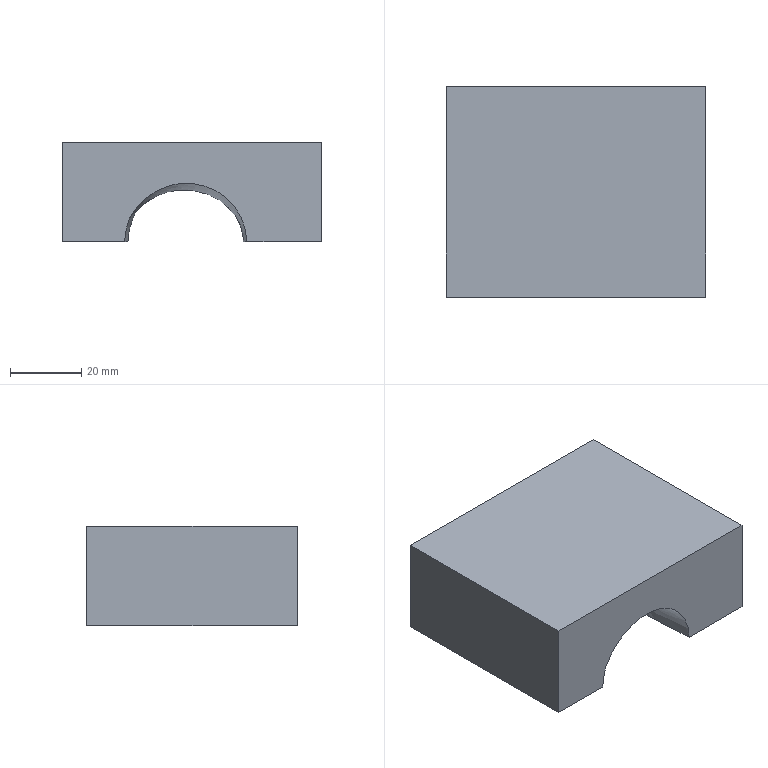Part | 1 solid | 22 faces | box 72.744 x 59.015 x 27.972 mm | volume 93773 mm3 | plane 11 | spline 7 | cylinder 4 | commonest cylinder face diameters 4.2 x2 6 x2